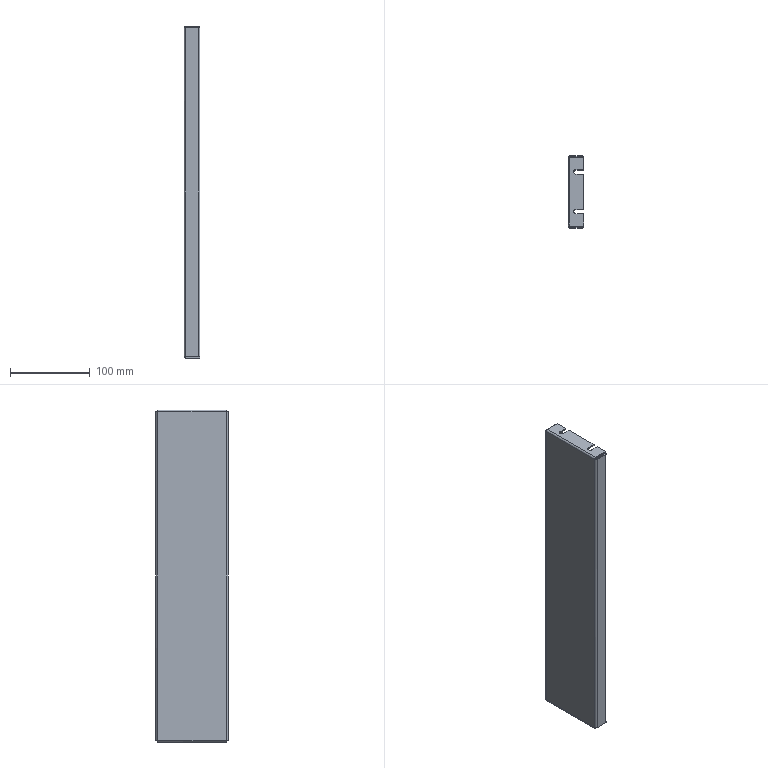Part | SolidWorks | features EdgeFlange 2, FlatPattern 1, HoleWzd 1, ICE 1, SMBaseFlange 1, SheetMetal 1 | 1 solid | 70 faces | box 20 x 90.5 x 416.5 mm | volume 94970 mm3 | plane 46 | cylinder 16 | spline 8 | commonest cylinder face diameters 1.473 x6 4.473 x6 5.8 x4